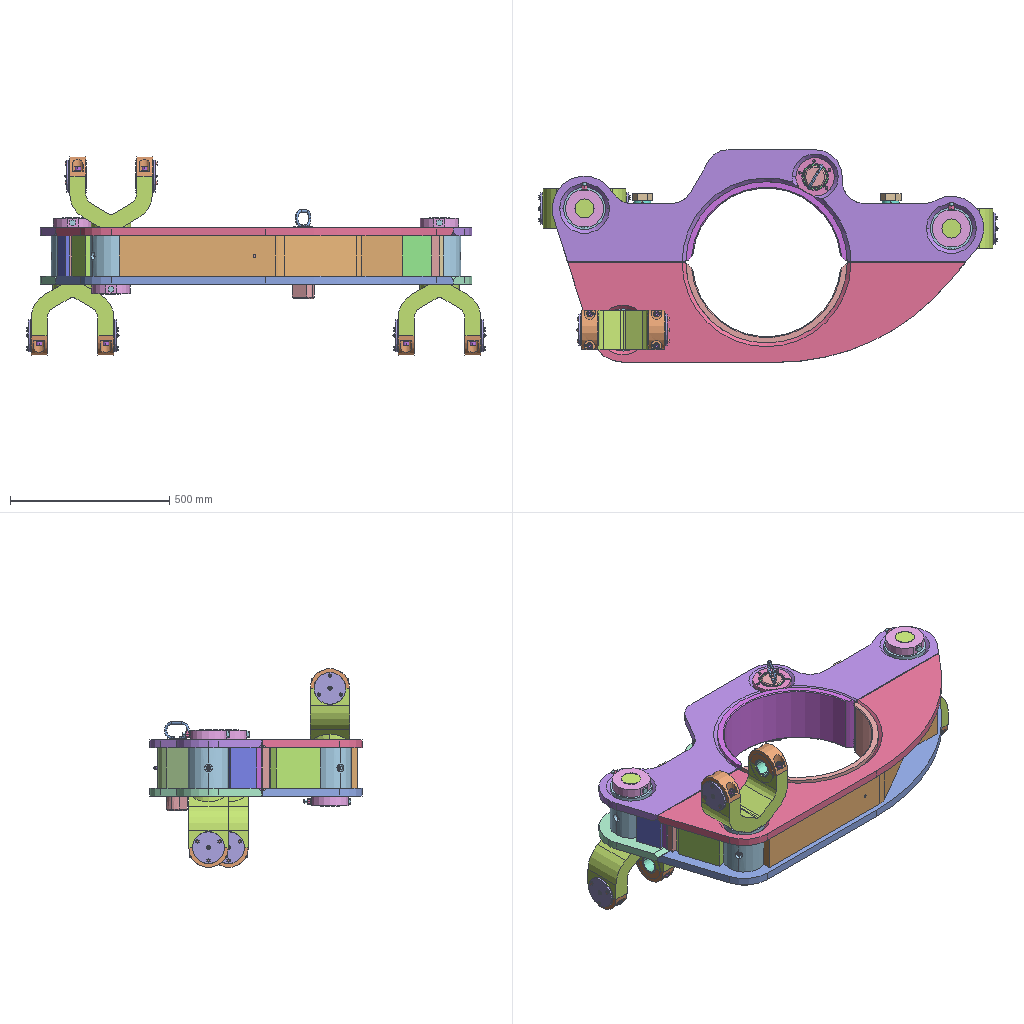Assembly | SolidWorks | 45 different items | 172 placed | box 1443 x 667 x 622 mm
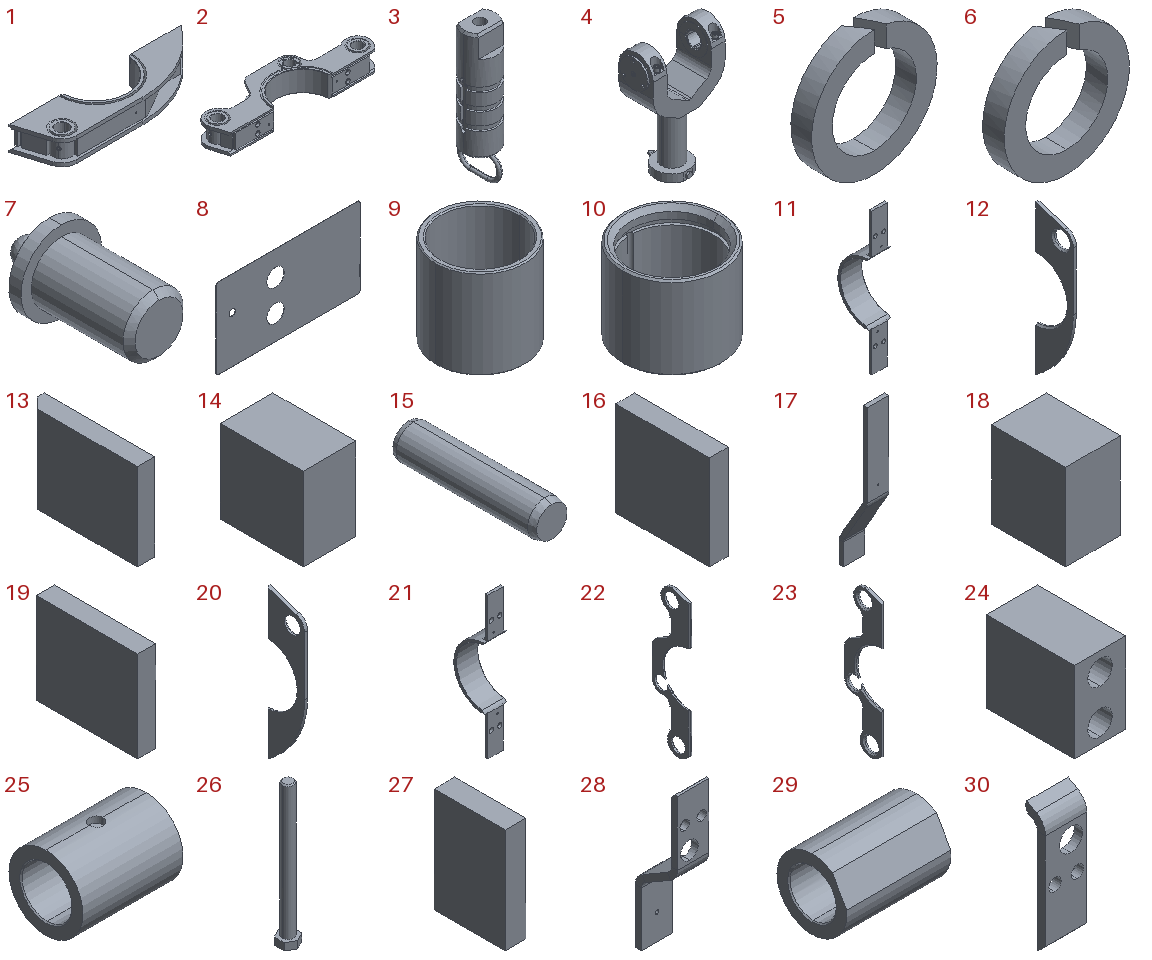Parts list (item | name | quantity | parent item | size | volume | features):
1 | (subassembly) | x1 | - | 1246 x 312.3 x 180 mm | 21895677 mm3 | features AEMSimFeature 1
2 | (subassembly) | x1 | - | 1354 x 352.3 x 180 mm | 22821153 mm3 | features AEMSimFeature 1, MirrorCompFeat 1, ReferencePattern 1
3 | (subassembly) | x1 | - | 70 x 90 x 279 mm | 792338 mm3 | -
4 | (subassembly) | x3 | - | 292 x 147.5 x 432 mm | 4101451 mm3 | features ReferencePattern 21, MirrorCompFeat 4, LocalCirPattern 1, LocalLPattern 1
5 | - | x4 | - | 54.5 x 9 x 54.5 mm | 11156 mm3 | features Extrusion 1, ICE 1
6 | - | x18 | in 4 | 9.3 x 1.6 x 9.3 mm | 59.55 mm3 | features Extrusion 1, ICE 1
7 | - | x10 | in 4 | 13.4 x 23.7 x 13.4 mm | 1610 mm3 | features Chamfer 1, Extrusion 1, ICE 1, Revolution 1
8 | - | x8 | - | 315 x 0.6 x 176 mm | 31798 mm3 | features Extrusion 1
9 | - | x2 | - | 80 x 80 x 80 mm | 93777 mm3 | features Chamfer 1, Extrusion 1
10 | - | x6 | - | 90 x 90 x 75 mm | 139007 mm3 | features Chamfer 2, ICE 2, Extrusion 1
11 | - | x1 | in 1 | 180 x 251.8 x 1160 mm | 4341383 mm3 | features ICE 4, Fillet 2, MirrorPattern 2, Chamfer 1, Extrusion 1, HoleWzd 1
12 | - | x1 | in 1 | 25 x 312.3 x 1246 mm | 4938572 mm3 | features Chamfer 2, Extrusion 1, Fillet 1, ICE 1
13 | - | x1 | in 1 | 25 x 160 x 126 mm | 489825 mm3 | features Chamfer 1, Extrusion 1
14 | - | x1 | in 1 | 80 x 126 x 126 mm | 1136246 mm3 | features Extrusion 1, HoleWzd 1
15 | - | x2 | - | 12 x 50 x 12 mm | 5242 mm3 | features Chamfer 2, Extrusion 1, HoleWzd 1
16 | - | x1 | in 1 | 25 x 125 x 126 mm | 393750 mm3 | features Extrusion 1
17 | - | x1 | in 1 | 126 x 168 x 887 mm | 2910198 mm3 | features FlatPattern 1, ICE 1, SMBaseFlange 1, SheetMetal 1
18 | - | x1 | in 1 | 80 x 108 x 126 mm | 954806 mm3 | features Extrusion 1, HoleWzd 1
19 | - | x1 | in 1 | 25 x 141 x 126 mm | 444150 mm3 | features Extrusion 1
20 | - | x1 | in 1 | 25 x 312.3 x 1246 mm | 4938572 mm3 | features Chamfer 2, Extrusion 1, Fillet 1, ICE 1
21 | - | x1 | in 2 | 180 x 251.8 x 1160 mm | 4313938 mm3 | features ICE 4, Fillet 2, MirrorPattern 2, Chamfer 1, Extrusion 1
22 | - | x1 | in 2 | 25 x 352.3 x 1354 mm | 4602346 mm3 | features ICE 3, Chamfer 2, Extrusion 1, Fillet 1
23 | - | x1 | in 2 | 25 x 352.3 x 1354 mm | 4602346 mm3 | features ICE 3, Chamfer 2, Extrusion 1, Fillet 1
24 | - | x2 | in 2 | 80 x 137 x 126 mm | 1070213 mm3 | features Extrusion 1
25 | - | x3 | in 1, 2 | 180 x 133 x 133 mm | 1348176 mm3 | features Chamfer 1, Extrusion 1, HoleWzd 1, ICE 1
26 | - | x3 | in 4 | 18 x 20.785 x 147.5 mm | 17913 mm3 | features Chamfer 1, Extrusion 1, ICE 1, RefAxis 1
27 | - | x1 | in 2 | 25 x 85.4 x 126 mm | 269010 mm3 | features Extrusion 1
28 | - | x1 | in 2 | 126 x 169.5 x 608 mm | 1978271 mm3 | features Chamfer 1, FlatPattern 1, HoleWzd 1, ICE 1, SMBaseFlange 1, SheetMetal 1
29 | - | x1 | in 2 | 180 x 121 x 121 mm | 1121817 mm3 | features HoleWzd 2, Chamfer 1, Extrusion 1, ICE 1
30 | - | x1 | in 2 | 126 x 61.5 x 380.651 mm | 1041526 mm3 | features Chamfer 2, FlatPattern 1, ICE 1, SMBaseFlange 1, SheetMetal 1
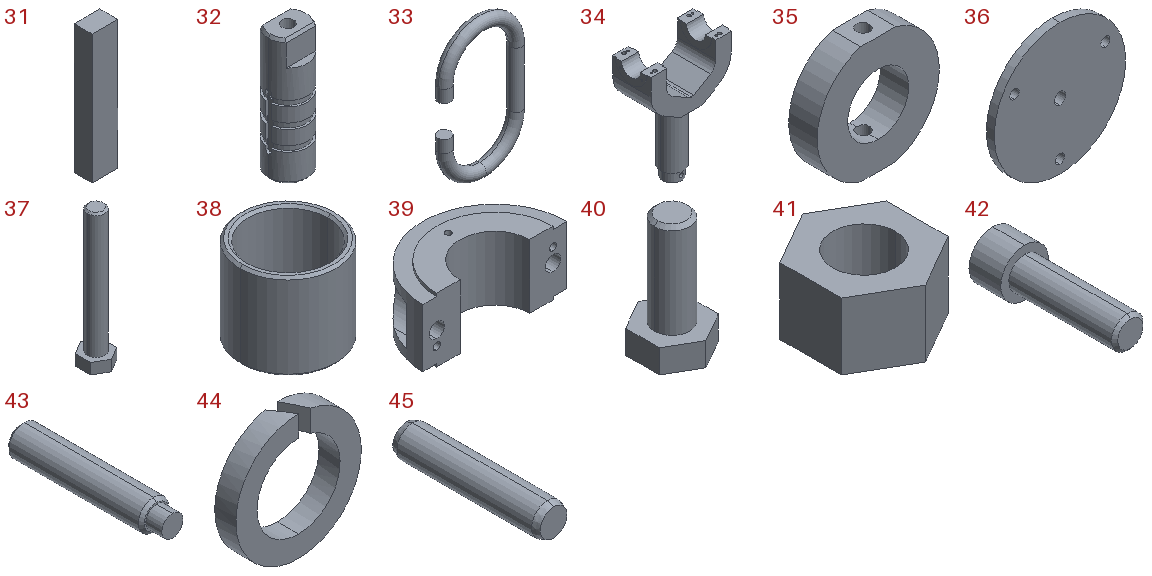31 | - | x1 | in 2 | 25 x 17.5 x 126 mm | 55125 mm3 | features Extrusion 1
32 | - | x1 | in 3 | 70 x 70 x 225 mm | 782460 mm3 | features ICE 6, Chamfer 3, Extrusion 1, HoleWzd 1, LPattern 1
33 | - | x1 | in 3 | 54 x 8 x 90 mm | 9878 mm3 | features Sweep 1
34 | - | x3 | in 4 | 265 x 124 x 370 mm | 3221545 mm3 | features ICE 7, HoleWzd 3, Chamfer 1, Extrusion 1, Fillet 1, MirrorPattern 1
35 | - | x3 | in 4 | 120 x 28 x 115 mm | 226944 mm3 | features ICE 2, Extrusion 1
36 | - | x6 | in 4 | 100 x 6 x 100 mm | 46049 mm3 | features Extrusion 1, HoleWzd 1, ICE 1
37 | - | x4 | - | 55 x 63.509 x 282.5 mm | 322908 mm3 | features Chamfer 1, Extrusion 1, ICE 1, RefAxis 1
38 | - | x6 | in 4 | 60 x 60 x 54 mm | 45325 mm3 | features Chamfer 1, Extrusion 1, ICE 1, RevCut 1
39 | - | x6 | in 4 | 124 x 62 x 55 mm | 204402 mm3 | features ICE 3, Extrusion 1, HoleWzd 1
40 | - | x18 | in 4 | 10 x 11.547 x 20 mm | 795.633 mm3 | features Chamfer 1, Extrusion 1, ICE 1, RefAxis 1
41 | - | x3 | in 4 | 17.3 x 19.976 x 10.8 mm | 1917 mm3 | features Extrusion 1, HoleWzd 1, RefAxis 1
42 | - | x12 | in 4 | 18 x 52 x 18 mm | 6970 mm3 | features ICE 2, Chamfer 1, Extrusion 1, RevCut 1
43 | - | x1 | - | 10 x 50 x 10 mm | 3601 mm3 | features ICE 3, Chamfer 1, Extrusion 1, RevCut 1
44 | - | x15 | in 4 | 18.4 x 3.1 x 18.4 mm | 445.195 mm3 | features Extrusion 1, ICE 1
45 | - | x12 | in 4 | 6 x 28 x 6 mm | 782.281 mm3 | features Chamfer 2, Extrusion 1
Mates (type | each side: item.copy, entity, surface, feature):
In the top assembly
Coincident | 1.1 plane | assembly plane | 3 times
DistanceDim | 8.1 plane | assembly plane
Coincident | 8.1 plane | assembly plane
Coincident | 12.1 face plane Boss-Extrude1 | 8.1 face plane Boss-Extrude1
DistanceDim | 8.2 plane | assembly plane
Coincident | 8.2 plane | assembly plane
Coincident | 12.1 face plane Boss-Extrude1 | 8.2 face plane Boss-Extrude1
Coincident | 2.1 plane | assembly plane | 3 times
Concentric | 29.1 face cylinder Boss-Extrude1 | 9.1 face cylinder Boss-Extrude1
Parallel | 9.1 plane | assembly plane
Coincident | 29.1 face plane Boss-Extrude1 | 9.1 face plane Boss-Extrude1
Perpendicular | 29.1 face plane Cut-Extrude1 | 3.1 plane
Concentric | 29.1 face cylinder Boss-Extrude1 | 32.1 face cylinder Boss-Extrude1
Concentric | 34.1 face cylinder Boss-Extrude3 | 25.1 face cylinder Boss-Extrude1
Parallel | 4.1 plane | assembly plane
Coincident | 25.1 face plane Boss-Extrude1 | 34.1 face plane Boss-Extrude1
Parallel | 10.1 plane | assembly plane
Concentric | 10.1 face cylinder Boss-Extrude1 | 25.1 face cylinder Boss-Extrude1
Coincident | 25.1 face plane Boss-Extrude1 | 10.1 face plane Boss-Extrude1
Coincident | 25.2 face plane Boss-Extrude1 | 34.2 face plane Boss-Extrude1
Concentric | 34.2 face cylinder Boss-Extrude3 | 25.2 face cylinder Boss-Extrude1
Parallel | 4.2 plane | assembly plane
Parallel | 10.2 plane | assembly plane
Coincident | 25.2 face plane Boss-Extrude1 | 10.2 face plane Boss-Extrude1
Concentric | 10.2 face cylinder Boss-Extrude1 | 25.2 face cylinder Boss-Extrude1
Coincident | 25.3 face plane Boss-Extrude1 | 34.3 face plane Boss-Extrude1
Concentric | 34.3 face cylinder Boss-Extrude3 | 25.3 face cylinder Boss-Extrude1
Parallel | 4.3 plane | assembly plane
Parallel | 10.3 plane | assembly plane
Coincident | 25.3 face plane Boss-Extrude1 | 10.3 face plane Boss-Extrude1
Concentric | 10.3 face cylinder Boss-Extrude1 | 25.3 face cylinder Boss-Extrude1
DistanceDim | 15.1 face plane Boss-Extrude1 | 1.1 plane
Concentric | 15.1 face cylinder Boss-Extrude1 | 11.1 face cylinder Cut-Extrude4
Parallel | 15.1 plane | assembly plane
DistanceDim | 15.2 face plane Boss-Extrude1 | 1.1 plane
Concentric | 11.1 face cylinder Cut-Extrude4 | 15.2 face cylinder Boss-Extrude1
Parallel | 15.2 plane | assembly plane
Parallel | 43.1 plane | assembly plane
DistanceDim | 29.1 face plane Boss-Extrude1 | 32.1 face plane Boss-Extrude1
Tangent | 32.1 face cylinder Cut-Extrude1 | 43.1 face plane Boss-Extrude2
Concentric | 29.1 face cylinder M10 Tapped Hole1 | 43.1 face cylinder Boss-Extrude1
Coincident | 28.1 face plane Base-Flange1 | 5.1 face plane Boss-Extrude1
Concentric | 5.1 face cylinder Boss-Extrude1 | 28.1 face cylinder Cut-Extrude2
Parallel | 5.1 plane | assembly plane
Coincident | 5.1 face plane Boss-Extrude1 | 37.1 face plane Boss-Extrude1
Parallel | 37.1 plane | assembly plane
Concentric | 37.1 face cylinder Boss-Extrude2 | 5.1 face cylinder Boss-Extrude1
Concentric | 32.1 face cylinder M10x1.0 Tapped Hole1 | 7.1 face cylinder Boss-Extrude2
Parallel | 7.1 plane | assembly plane
Coincident | 32.1 face plane Cut-Extrude5 | 7.1 face plane Boss-Extrude1
Concentric | 7.2 face cylinder Boss-Extrude2 | 25.1 face cylinder Cut-Extrude1
Parallel | 7.2 plane | assembly plane
Coincident | 25.1 face plane Cut-Extrude1 | 7.2 face plane Boss-Extrude1
Concentric | 7.3 face cylinder Boss-Extrude2 | 25.2 face cylinder Cut-Extrude1
Parallel | 7.3 plane | assembly plane
Coincident | 25.2 face plane Cut-Extrude1 | 7.3 face plane Boss-Extrude1
Concentric | 7.4 face cylinder Boss-Extrude2 | 25.3 face cylinder Cut-Extrude1
Parallel | 7.4 plane | assembly plane
Coincident | 25.3 face plane Cut-Extrude1 | 7.4 face plane Boss-Extrude1
In subassembly 3
Tangent | 32.2 face plane Boss-Extrude1 | 33.1 face cylinder Sweep1
Coincident | 32.2 plane | 33.1 plane | 2 times
Coincident | 32.2 plane | 3.2 plane | 3 times
In subassembly 4
Coincident | 34.4 axis | 35.1 axis | 2 times
Coincident | 34.4 axis | 38.1 axis
PlanarAngleDim | 38.1 plane | 34.4 face plane Boss-Extrude1
Coincident | 34.4 face plane Boss-Extrude5 | 38.1 face plane Boss-Extrude1
Coincident | 34.4 axis | 39.1 axis | 3 times
Coincident | 34.4 axis | 39.2 axis | 3 times
Coincident | 34.4 plane | 4.4 plane | 3 times
Parallel | 44.1 plane | 4.4 plane
Coincident | 35.1 axis | 44.1 axis
Coincident | 35.1 face plane Cut-Extrude1 | 44.1 face plane Boss-Extrude1
Parallel | 41.1 plane | 4.4 plane
Coincident | 44.1 face plane Boss-Extrude1 | 41.1 face plane Boss-Extrude1
Coincident | 35.1 axis | 41.1 axis
Parallel | 26.1 plane | 4.4 plane
Coincident | 35.1 axis | 26.1 axis
Coincident | 35.1 face plane Cut-Extrude1 | 26.1 face plane Boss-Extrude1
Coincident | 34.4 axis | 45.1 axis
Coincident | 34.4 face plane Boss-Extrude1 | 45.1 plane
Parallel | 45.1 plane | 4.4 plane
Coincident | 34.4 face plane Boss-Extrude1 | 45.2 plane
Coincident | 34.4 axis | 45.2 axis
Parallel | 45.2 plane | 4.4 plane
Parallel | 44.2 plane | 4.4 plane
Coincident | 39.1 face plane Cut-Extrude1 | 44.2 face plane Boss-Extrude1
Coincident | 39.1 axis | 44.2 axis
Coincident | 44.2 face plane Boss-Extrude1 | 42.1 face plane Boss-Extrude1
Parallel | 42.1 plane | 4.4 plane
Coincident | 39.1 axis | 42.1 axis
Coincident | 36.1 face plane Boss-Extrude1 | 6.1 face plane Boss-Extrude1
Parallel | 6.1 plane | 4.4 plane
Coincident | 36.1 axis | 6.1 axis
Coincident | 36.1 axis | 40.1 axis
Parallel | 40.1 plane | 4.4 plane
Coincident | 6.1 face plane Boss-Extrude1 | 40.1 face plane Boss-Extrude1
Coincident | 36.1 axis | 7.1 axis
Parallel | 7.1 plane | 4.4 plane
Coincident | 36.1 face plane Boss-Extrude1 | 7.1 face plane Boss-Extrude1
Coincident | 34.4 face plane Boss-Extrude5 | 36.1 face plane Boss-Extrude1
Concentric | 34.4 face cylinder Mirror1 | 36.1 face cylinder Cut-Extrude1 | 2 times
In subassembly 2
Coincident | 21.1 plane | 2.2 plane | 3 times
DistanceDim | 23.1 face plane Boss-Extrude1 | 2.2 plane
Coincident | 23.1 plane | 2.2 plane | 2 times
DistanceDim | 24.1 plane | 2.2 plane
DistanceDim | 24.1 face plane Boss-Extrude1 | 2.2 plane
Parallel | 25.4 plane | 2.2 plane
Coincident | 25.4 plane | 2.2 plane
Parallel | 25.5 plane | 2.2 plane
Coincident | 27.1 plane | 2.2 plane
Coincident | 23.1 face plane Boss-Extrude1 | 28.2 face plane Base-Flange1
Coincident | 23.1 face plane Boss-Extrude1 | 30.1 face plane Base-Flange1
DistanceDim | 31.1 face plane Boss-Extrude1 | 2.2 plane
Coincident | 22.1 plane | 2.2 plane | 2 times
Coincident | 24.1 plane | 2.2 plane
Concentric | 23.1 face cylinder Cut-Extrude1 | 25.4 face cylinder Boss-Extrude1
Concentric | 23.1 face cylinder Cut-Extrude1 | 25.5 face cylinder Boss-Extrude1
Coincident | 25.5 plane | 2.2 plane
Tangent | 25.4 face cylinder Boss-Extrude1 | 27.1 edge
DistanceDim | 27.1 face plane Boss-Extrude1 | 23.1 face plane Boss-Extrude1
Coincident | 28.2 plane | 2.2 plane
DistanceDim | 28.2 plane | 2.2 plane
Concentric | 23.1 face cylinder Cut-Extrude1 | 29.2 face cylinder Boss-Extrude1
Parallel | 29.2 plane | 2.2 plane
Coincident | 29.2 plane | 2.2 plane
DistanceDim | 30.1 plane | 2.2 plane
Coincident | 30.1 plane | 2.2 plane
Coincident | 31.1 plane | 2.2 plane
DistanceDim | 31.1 plane | 2.2 plane
DistanceDim | 22.1 face plane Boss-Extrude1 | 2.2 plane
In subassembly 1
Coincident | 11.2 plane | 1.2 plane | 3 times
Coincident | 11.2 face plane Boss-Extrude1 | 13.1 edge
Coincident | 13.1 plane | 1.2 plane
DistanceDim | 14.1 plane | 1.2 plane
Coincident | 11.2 face plane Boss-Extrude1 | 14.1 face plane Boss-Extrude1
DistanceDim | 16.1 face plane Boss-Extrude1 | 1.2 plane
Coincident | 17.1 plane | 1.2 plane | 2 times
DistanceDim | 18.1 plane | 1.2 plane
Coincident | 11.2 face plane Boss-Extrude1 | 18.1 face plane Boss-Extrude1
Coincident | 11.2 face plane Boss-Extrude1 | 19.1 edge
Coincident | 19.1 plane | 1.2 plane
DistanceDim | 1.2 plane | 20.1 face plane Boss-Extrude1
Coincident | 20.1 plane | 1.2 plane | 2 times
PlanarAngleDim | 25.4 plane | 1.2 plane
DistanceDim | 12.2 face plane Boss-Extrude1 | 1.2 plane
Coincident | 12.2 plane | 1.2 plane | 2 times
DistanceDim | 13.1 face plane Boss-Extrude1 | 12.2 face plane Boss-Extrude1
Coincident | 14.1 plane | 1.2 plane
Coincident | 16.1 plane | 1.2 plane
Coincident | 14.1 face plane Boss-Extrude1 | 16.1 face plane Boss-Extrude1
Coincident | 16.1 face plane Boss-Extrude1 | 17.1 face plane Base-Flange1
Coincident | 18.1 plane | 1.2 plane
Coincident | 18.1 face plane Boss-Extrude1 | 19.1 edge
Coincident | 17.1 face plane Base-Flange1 | 19.1 edge
Coincident | 25.4 plane | 1.2 plane
Concentric | 12.2 face cylinder Cut-Extrude1 | 25.4 face cylinder Boss-Extrude1